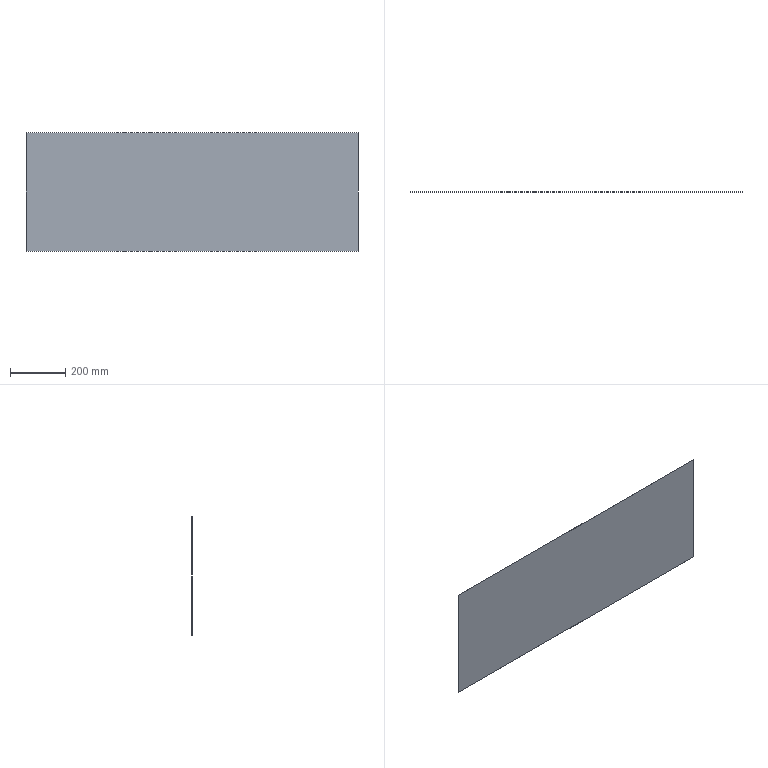Part | STEP file | Polyester film | 1 solid | 6 faces | box 1200 x 0.25 x 430 mm | volume 129000 mm3 | plane 6
STEP:
#1=CARTESIAN_POINT('',(0.,0.,0.));
#2=DIRECTION('',(0.,0.,1.));
#3=DIRECTION('',(1.,0.,0.));
#4=AXIS2_PLACEMENT_3D('',#1,#2,#3);
#5=CARTESIAN_POINT('',(600.,0.25,-215.));
#6=VERTEX_POINT('',#5);
#7=CARTESIAN_POINT('',(-600.,0.25,-215.));
#8=VERTEX_POINT('',#7);
#9=CARTESIAN_POINT('',(-600.,0.25,-215.));
#10=DIRECTION('',(-1.,0.,0.));
#11=VECTOR('',#10,1.);
#12=LINE('',#9,#11);
#13=CARTESIAN_POINT('',(-600.,0.25,215.));
#14=DIRECTION('',(0.,-1.,0.));
#15=DIRECTION('',(0.,0.,-1.));
#16=AXIS2_PLACEMENT_3D('',#13,#14,#15);
#17=PLANE('',#16);
#18=CARTESIAN_POINT('',(430.,0.));
#19=DIRECTION('',(0.,-1.));
#20=VECTOR('',#19,1.);
#21=LINE('',#18,#20);
#22=(GEOMETRIC_REPRESENTATION_CONTEXT(2)PARAMETRIC_REPRESENTATION_CONTEXT()REPRESENTATION_CONTEXT('',''));
#23=DEFINITIONAL_REPRESENTATION('',(#21),#22);
#24=PCURVE('',#17,#23);
#25=CARTESIAN_POINT('',(-600.,0.25,-215.));
#26=DIRECTION('',(0.,0.,1.));
#27=DIRECTION('',(1.,0.,0.));
#28=AXIS2_PLACEMENT_3D('',#25,#26,#27);
#29=PLANE('',#28);
#30=CARTESIAN_POINT('',(0.,0.));
#31=DIRECTION('',(-1.,0.));
#32=VECTOR('',#31,1.);
#33=LINE('',#30,#32);
#34=(GEOMETRIC_REPRESENTATION_CONTEXT(2)PARAMETRIC_REPRESENTATION_CONTEXT()REPRESENTATION_CONTEXT('',''));
#35=DEFINITIONAL_REPRESENTATION('',(#33),#34);
#36=PCURVE('',#29,#35);
#37=SURFACE_CURVE('',#12,(#24,#36),.PCURVE_S1.);
#38=EDGE_CURVE('',#6,#8,#37,.T.);
#39=ORIENTED_EDGE('',*,*,#38,.T.);
#40=CARTESIAN_POINT('',(-600.,0.25,215.));
#41=VERTEX_POINT('',#40);
#42=CARTESIAN_POINT('',(-600.,0.25,215.));
#43=DIRECTION('',(0.,0.,-1.));
#44=VECTOR('',#43,1.);
#45=LINE('',#42,#44);
#46=CARTESIAN_POINT('',(0.,0.));
#47=DIRECTION('',(1.,0.));
#48=VECTOR('',#47,1.);
#49=LINE('',#46,#48);
#50=(GEOMETRIC_REPRESENTATION_CONTEXT(2)PARAMETRIC_REPRESENTATION_CONTEXT()REPRESENTATION_CONTEXT('',''));
#51=DEFINITIONAL_REPRESENTATION('',(#49),#50);
#52=PCURVE('',#17,#51);
#53=CARTESIAN_POINT('',(-600.,0.,215.));
#54=DIRECTION('',(-1.,0.,0.));
#55=DIRECTION('',(0.,0.,1.));
#56=AXIS2_PLACEMENT_3D('',#53,#54,#55);
#57=PLANE('',#56);
#58=CARTESIAN_POINT('',(0.,0.25));
#59=DIRECTION('',(-1.,0.));
#60=VECTOR('',#59,1.);
#61=LINE('',#58,#60);
#62=(GEOMETRIC_REPRESENTATION_CONTEXT(2)PARAMETRIC_REPRESENTATION_CONTEXT()REPRESENTATION_CONTEXT('',''));
#63=DEFINITIONAL_REPRESENTATION('',(#61),#62);
#64=PCURVE('',#57,#63);
#65=SURFACE_CURVE('',#45,(#52,#64),.PCURVE_S1.);
#66=EDGE_CURVE('',#41,#8,#65,.T.);
#67=ORIENTED_EDGE('',*,*,#66,.F.);
#68=CARTESIAN_POINT('',(600.,0.25,215.));
#69=VERTEX_POINT('',#68);
#70=CARTESIAN_POINT('',(-600.,0.25,215.));
#71=DIRECTION('',(-1.,0.,0.));
#72=VECTOR('',#71,1.);
#73=LINE('',#70,#72);
#74=CARTESIAN_POINT('',(0.,0.));
#75=DIRECTION('',(0.,-1.));
#76=VECTOR('',#75,1.);
#77=LINE('',#74,#76);
#78=(GEOMETRIC_REPRESENTATION_CONTEXT(2)PARAMETRIC_REPRESENTATION_CONTEXT()REPRESENTATION_CONTEXT('',''));
#79=DEFINITIONAL_REPRESENTATION('',(#77),#78);
#80=PCURVE('',#17,#79);
#81=CARTESIAN_POINT('',(-600.,0.25,215.));
#82=DIRECTION('',(0.,0.,1.));
#83=DIRECTION('',(1.,0.,0.));
#84=AXIS2_PLACEMENT_3D('',#81,#82,#83);
#85=PLANE('',#84);
#86=CARTESIAN_POINT('',(0.,0.));
#87=DIRECTION('',(-1.,0.));
#88=VECTOR('',#87,1.);
#89=LINE('',#86,#88);
#90=(GEOMETRIC_REPRESENTATION_CONTEXT(2)PARAMETRIC_REPRESENTATION_CONTEXT()REPRESENTATION_CONTEXT('',''));
#91=DEFINITIONAL_REPRESENTATION('',(#89),#90);
#92=PCURVE('',#85,#91);
#93=SURFACE_CURVE('',#73,(#80,#92),.PCURVE_S1.);
#94=EDGE_CURVE('',#69,#41,#93,.T.);
#95=ORIENTED_EDGE('',*,*,#94,.F.);
#96=CARTESIAN_POINT('',(600.,0.25,215.));
#97=DIRECTION('',(0.,0.,-1.));
#98=VECTOR('',#97,1.);
#99=LINE('',#96,#98);
#100=CARTESIAN_POINT('',(0.,1200.));
#101=DIRECTION('',(1.,0.));
#102=VECTOR('',#101,1.);
#103=LINE('',#100,#102);
#104=(GEOMETRIC_REPRESENTATION_CONTEXT(2)PARAMETRIC_REPRESENTATION_CONTEXT()REPRESENTATION_CONTEXT('',''));
#105=DEFINITIONAL_REPRESENTATION('',(#103),#104);
#106=PCURVE('',#17,#105);
#107=CARTESIAN_POINT('',(600.,0.25,215.));
#108=DIRECTION('',(1.,0.,0.));
#109=DIRECTION('',(0.,0.,-1.));
#110=AXIS2_PLACEMENT_3D('',#107,#108,#109);
#111=PLANE('',#110);
#112=CARTESIAN_POINT('',(0.,0.));
#113=DIRECTION('',(1.,0.));
#114=VECTOR('',#113,1.);
#115=LINE('',#112,#114);
#116=(GEOMETRIC_REPRESENTATION_CONTEXT(2)PARAMETRIC_REPRESENTATION_CONTEXT()REPRESENTATION_CONTEXT('',''));
#117=DEFINITIONAL_REPRESENTATION('',(#115),#116);
#118=PCURVE('',#111,#117);
#119=SURFACE_CURVE('',#99,(#106,#118),.PCURVE_S1.);
#120=EDGE_CURVE('',#69,#6,#119,.T.);
#121=ORIENTED_EDGE('',*,*,#120,.T.);
#122=EDGE_LOOP('',(#39,#67,#95,#121));
#123=FACE_BOUND('',#122,.T.);
#124=ADVANCED_FACE('',(#123),#17,.F.);
#125=CARTESIAN_POINT('',(-600.,0.,-215.));
#126=VERTEX_POINT('',#125);
#127=CARTESIAN_POINT('',(-600.,0.,-215.));
#128=DIRECTION('',(0.,1.,0.));
#129=VECTOR('',#128,1.);
#130=LINE('',#127,#129);
#131=CARTESIAN_POINT('',(-430.,0.));
#132=DIRECTION('',(0.,1.));
#133=VECTOR('',#132,1.);
#134=LINE('',#131,#133);
#135=(GEOMETRIC_REPRESENTATION_CONTEXT(2)PARAMETRIC_REPRESENTATION_CONTEXT()REPRESENTATION_CONTEXT('',''));
#136=DEFINITIONAL_REPRESENTATION('',(#134),#135);
#137=PCURVE('',#57,#136);
#138=CARTESIAN_POINT('',(0.,-0.25));
#139=DIRECTION('',(0.,1.));
#140=VECTOR('',#139,1.);
#141=LINE('',#138,#140);
#142=(GEOMETRIC_REPRESENTATION_CONTEXT(2)PARAMETRIC_REPRESENTATION_CONTEXT()REPRESENTATION_CONTEXT('',''));
#143=DEFINITIONAL_REPRESENTATION('',(#141),#142);
#144=PCURVE('',#29,#143);
#145=SURFACE_CURVE('',#130,(#137,#144),.PCURVE_S1.);
#146=EDGE_CURVE('',#126,#8,#145,.T.);
#147=ORIENTED_EDGE('',*,*,#146,.F.);
#148=CARTESIAN_POINT('',(-600.,0.,215.));
#149=VERTEX_POINT('',#148);
#150=CARTESIAN_POINT('',(-600.,0.,215.));
#151=DIRECTION('',(0.,0.,-1.));
#152=VECTOR('',#151,1.);
#153=LINE('',#150,#152);
#154=CARTESIAN_POINT('',(0.,0.));
#155=DIRECTION('',(-1.,0.));
#156=VECTOR('',#155,1.);
#157=LINE('',#154,#156);
#158=(GEOMETRIC_REPRESENTATION_CONTEXT(2)PARAMETRIC_REPRESENTATION_CONTEXT()REPRESENTATION_CONTEXT('',''));
#159=DEFINITIONAL_REPRESENTATION('',(#157),#158);
#160=PCURVE('',#57,#159);
#161=CARTESIAN_POINT('',(-600.,0.,215.));
#162=DIRECTION('',(0.,-1.,0.));
#163=DIRECTION('',(0.,0.,-1.));
#164=AXIS2_PLACEMENT_3D('',#161,#162,#163);
#165=PLANE('',#164);
#166=CARTESIAN_POINT('',(0.,0.));
#167=DIRECTION('',(1.,0.));
#168=VECTOR('',#167,1.);
#169=LINE('',#166,#168);
#170=(GEOMETRIC_REPRESENTATION_CONTEXT(2)PARAMETRIC_REPRESENTATION_CONTEXT()REPRESENTATION_CONTEXT('',''));
#171=DEFINITIONAL_REPRESENTATION('',(#169),#170);
#172=PCURVE('',#165,#171);
#173=SURFACE_CURVE('',#153,(#160,#172),.PCURVE_S1.);
#174=EDGE_CURVE('',#149,#126,#173,.T.);
#175=ORIENTED_EDGE('',*,*,#174,.F.);
#176=CARTESIAN_POINT('',(-600.,0.,215.));
#177=DIRECTION('',(0.,1.,0.));
#178=VECTOR('',#177,1.);
#179=LINE('',#176,#178);
#180=CARTESIAN_POINT('',(0.,0.));
#181=DIRECTION('',(0.,1.));
#182=VECTOR('',#181,1.);
#183=LINE('',#180,#182);
#184=(GEOMETRIC_REPRESENTATION_CONTEXT(2)PARAMETRIC_REPRESENTATION_CONTEXT()REPRESENTATION_CONTEXT('',''));
#185=DEFINITIONAL_REPRESENTATION('',(#183),#184);
#186=PCURVE('',#57,#185);
#187=CARTESIAN_POINT('',(0.,-0.25));
#188=DIRECTION('',(0.,1.));
#189=VECTOR('',#188,1.);
#190=LINE('',#187,#189);
#191=(GEOMETRIC_REPRESENTATION_CONTEXT(2)PARAMETRIC_REPRESENTATION_CONTEXT()REPRESENTATION_CONTEXT('',''));
#192=DEFINITIONAL_REPRESENTATION('',(#190),#191);
#193=PCURVE('',#85,#192);
#194=SURFACE_CURVE('',#179,(#186,#193),.PCURVE_S1.);
#195=EDGE_CURVE('',#149,#41,#194,.T.);
#196=ORIENTED_EDGE('',*,*,#195,.T.);
#197=ORIENTED_EDGE('',*,*,#66,.T.);
#198=EDGE_LOOP('',(#147,#175,#196,#197));
#199=FACE_BOUND('',#198,.T.);
#200=ADVANCED_FACE('',(#199),#57,.T.);
#201=CARTESIAN_POINT('',(600.,0.,-215.));
#202=VERTEX_POINT('',#201);
#203=CARTESIAN_POINT('',(-600.,0.,-215.));
#204=DIRECTION('',(-1.,0.,0.));
#205=VECTOR('',#204,1.);
#206=LINE('',#203,#205);
#207=CARTESIAN_POINT('',(430.,0.));
#208=DIRECTION('',(0.,-1.));
#209=VECTOR('',#208,1.);
#210=LINE('',#207,#209);
#211=(GEOMETRIC_REPRESENTATION_CONTEXT(2)PARAMETRIC_REPRESENTATION_CONTEXT()REPRESENTATION_CONTEXT('',''));
#212=DEFINITIONAL_REPRESENTATION('',(#210),#211);
#213=PCURVE('',#165,#212);
#214=CARTESIAN_POINT('',(0.,-0.25));
#215=DIRECTION('',(-1.,0.));
#216=VECTOR('',#215,1.);
#217=LINE('',#214,#216);
#218=(GEOMETRIC_REPRESENTATION_CONTEXT(2)PARAMETRIC_REPRESENTATION_CONTEXT()REPRESENTATION_CONTEXT('',''));
#219=DEFINITIONAL_REPRESENTATION('',(#217),#218);
#220=PCURVE('',#29,#219);
#221=SURFACE_CURVE('',#206,(#213,#220),.PCURVE_S1.);
#222=EDGE_CURVE('',#202,#126,#221,.T.);
#223=ORIENTED_EDGE('',*,*,#222,.F.);
#224=CARTESIAN_POINT('',(600.,0.,215.));
#225=VERTEX_POINT('',#224);
#226=CARTESIAN_POINT('',(600.,0.,215.));
#227=DIRECTION('',(0.,0.,-1.));
#228=VECTOR('',#227,1.);
#229=LINE('',#226,#228);
#230=CARTESIAN_POINT('',(0.,1200.));
#231=DIRECTION('',(1.,0.));
#232=VECTOR('',#231,1.);
#233=LINE('',#230,#232);
#234=(GEOMETRIC_REPRESENTATION_CONTEXT(2)PARAMETRIC_REPRESENTATION_CONTEXT()REPRESENTATION_CONTEXT('',''));
#235=DEFINITIONAL_REPRESENTATION('',(#233),#234);
#236=PCURVE('',#165,#235);
#237=CARTESIAN_POINT('',(0.,-0.25));
#238=DIRECTION('',(1.,0.));
#239=VECTOR('',#238,1.);
#240=LINE('',#237,#239);
#241=(GEOMETRIC_REPRESENTATION_CONTEXT(2)PARAMETRIC_REPRESENTATION_CONTEXT()REPRESENTATION_CONTEXT('',''));
#242=DEFINITIONAL_REPRESENTATION('',(#240),#241);
#243=PCURVE('',#111,#242);
#244=SURFACE_CURVE('',#229,(#236,#243),.PCURVE_S1.);
#245=EDGE_CURVE('',#225,#202,#244,.T.);
#246=ORIENTED_EDGE('',*,*,#245,.F.);
#247=CARTESIAN_POINT('',(-600.,0.,215.));
#248=DIRECTION('',(-1.,0.,0.));
#249=VECTOR('',#248,1.);
#250=LINE('',#247,#249);
#251=CARTESIAN_POINT('',(0.,0.));
#252=DIRECTION('',(0.,-1.));
#253=VECTOR('',#252,1.);
#254=LINE('',#251,#253);
#255=(GEOMETRIC_REPRESENTATION_CONTEXT(2)PARAMETRIC_REPRESENTATION_CONTEXT()REPRESENTATION_CONTEXT('',''));
#256=DEFINITIONAL_REPRESENTATION('',(#254),#255);
#257=PCURVE('',#165,#256);
#258=CARTESIAN_POINT('',(0.,-0.25));
#259=DIRECTION('',(-1.,0.));
#260=VECTOR('',#259,1.);
#261=LINE('',#258,#260);
#262=(GEOMETRIC_REPRESENTATION_CONTEXT(2)PARAMETRIC_REPRESENTATION_CONTEXT()REPRESENTATION_CONTEXT('',''));
#263=DEFINITIONAL_REPRESENTATION('',(#261),#262);
#264=PCURVE('',#85,#263);
#265=SURFACE_CURVE('',#250,(#257,#264),.PCURVE_S1.);
#266=EDGE_CURVE('',#225,#149,#265,.T.);
#267=ORIENTED_EDGE('',*,*,#266,.T.);
#268=ORIENTED_EDGE('',*,*,#174,.T.);
#269=EDGE_LOOP('',(#223,#246,#267,#268));
#270=FACE_BOUND('',#269,.T.);
#271=ADVANCED_FACE('',(#270),#165,.T.);
#272=CARTESIAN_POINT('',(600.,0.25,-215.));
#273=DIRECTION('',(0.,-1.,0.));
#274=VECTOR('',#273,1.);
#275=LINE('',#272,#274);
#276=CARTESIAN_POINT('',(430.,0.));
#277=DIRECTION('',(0.,-1.));
#278=VECTOR('',#277,1.);
#279=LINE('',#276,#278);
#280=(GEOMETRIC_REPRESENTATION_CONTEXT(2)PARAMETRIC_REPRESENTATION_CONTEXT()REPRESENTATION_CONTEXT('',''));
#281=DEFINITIONAL_REPRESENTATION('',(#279),#280);
#282=PCURVE('',#111,#281);
#283=CARTESIAN_POINT('',(1200.,0.));
#284=DIRECTION('',(0.,-1.));
#285=VECTOR('',#284,1.);
#286=LINE('',#283,#285);
#287=(GEOMETRIC_REPRESENTATION_CONTEXT(2)PARAMETRIC_REPRESENTATION_CONTEXT()REPRESENTATION_CONTEXT('',''));
#288=DEFINITIONAL_REPRESENTATION('',(#286),#287);
#289=PCURVE('',#29,#288);
#290=SURFACE_CURVE('',#275,(#282,#289),.PCURVE_S1.);
#291=EDGE_CURVE('',#6,#202,#290,.T.);
#292=ORIENTED_EDGE('',*,*,#291,.F.);
#293=ORIENTED_EDGE('',*,*,#120,.F.);
#294=CARTESIAN_POINT('',(600.,0.25,215.));
#295=DIRECTION('',(0.,-1.,0.));
#296=VECTOR('',#295,1.);
#297=LINE('',#294,#296);
#298=CARTESIAN_POINT('',(0.,0.));
#299=DIRECTION('',(0.,-1.));
#300=VECTOR('',#299,1.);
#301=LINE('',#298,#300);
#302=(GEOMETRIC_REPRESENTATION_CONTEXT(2)PARAMETRIC_REPRESENTATION_CONTEXT()REPRESENTATION_CONTEXT('',''));
#303=DEFINITIONAL_REPRESENTATION('',(#301),#302);
#304=PCURVE('',#111,#303);
#305=CARTESIAN_POINT('',(1200.,0.));
#306=DIRECTION('',(0.,-1.));
#307=VECTOR('',#306,1.);
#308=LINE('',#305,#307);
#309=(GEOMETRIC_REPRESENTATION_CONTEXT(2)PARAMETRIC_REPRESENTATION_CONTEXT()REPRESENTATION_CONTEXT('',''));
#310=DEFINITIONAL_REPRESENTATION('',(#308),#309);
#311=PCURVE('',#85,#310);
#312=SURFACE_CURVE('',#297,(#304,#311),.PCURVE_S1.);
#313=EDGE_CURVE('',#69,#225,#312,.T.);
#314=ORIENTED_EDGE('',*,*,#313,.T.);
#315=ORIENTED_EDGE('',*,*,#245,.T.);
#316=EDGE_LOOP('',(#292,#293,#314,#315));
#317=FACE_BOUND('',#316,.T.);
#318=ADVANCED_FACE('',(#317),#111,.T.);
#319=ORIENTED_EDGE('',*,*,#94,.T.);
#320=ORIENTED_EDGE('',*,*,#195,.F.);
#321=ORIENTED_EDGE('',*,*,#266,.F.);
#322=ORIENTED_EDGE('',*,*,#313,.F.);
#323=EDGE_LOOP('',(#319,#320,#321,#322));
#324=FACE_BOUND('',#323,.T.);
#325=ADVANCED_FACE('',(#324),#85,.T.);
#326=ORIENTED_EDGE('',*,*,#38,.F.);
#327=ORIENTED_EDGE('',*,*,#291,.T.);
#328=ORIENTED_EDGE('',*,*,#222,.T.);
#329=ORIENTED_EDGE('',*,*,#146,.T.);
#330=EDGE_LOOP('',(#326,#327,#328,#329));
#331=FACE_BOUND('',#330,.T.);
#332=ADVANCED_FACE('',(#331),#29,.F.);
#333=CLOSED_SHELL('',(#124,#200,#271,#318,#325,#332));
#334=MANIFOLD_SOLID_BREP('',#333);
#335=(LENGTH_UNIT()NAMED_UNIT(*)SI_UNIT(.MILLI.,.METRE.));
#336=UNCERTAINTY_MEASURE_WITH_UNIT(LENGTH_MEASURE(0.0000001),#335,'','');
#337=(NAMED_UNIT(*)PLANE_ANGLE_UNIT()SI_UNIT($,.RADIAN.));
#338=(NAMED_UNIT(*)SI_UNIT($,.STERADIAN.)SOLID_ANGLE_UNIT());
#339=(GEOMETRIC_REPRESENTATION_CONTEXT(3)GLOBAL_UNCERTAINTY_ASSIGNED_CONTEXT((#336))GLOBAL_UNIT_ASSIGNED_CONTEXT((#335,#337,#338))REPRESENTATION_CONTEXT('',''));
#340=ADVANCED_BREP_SHAPE_REPRESENTATION('',(#4,#334),#339);